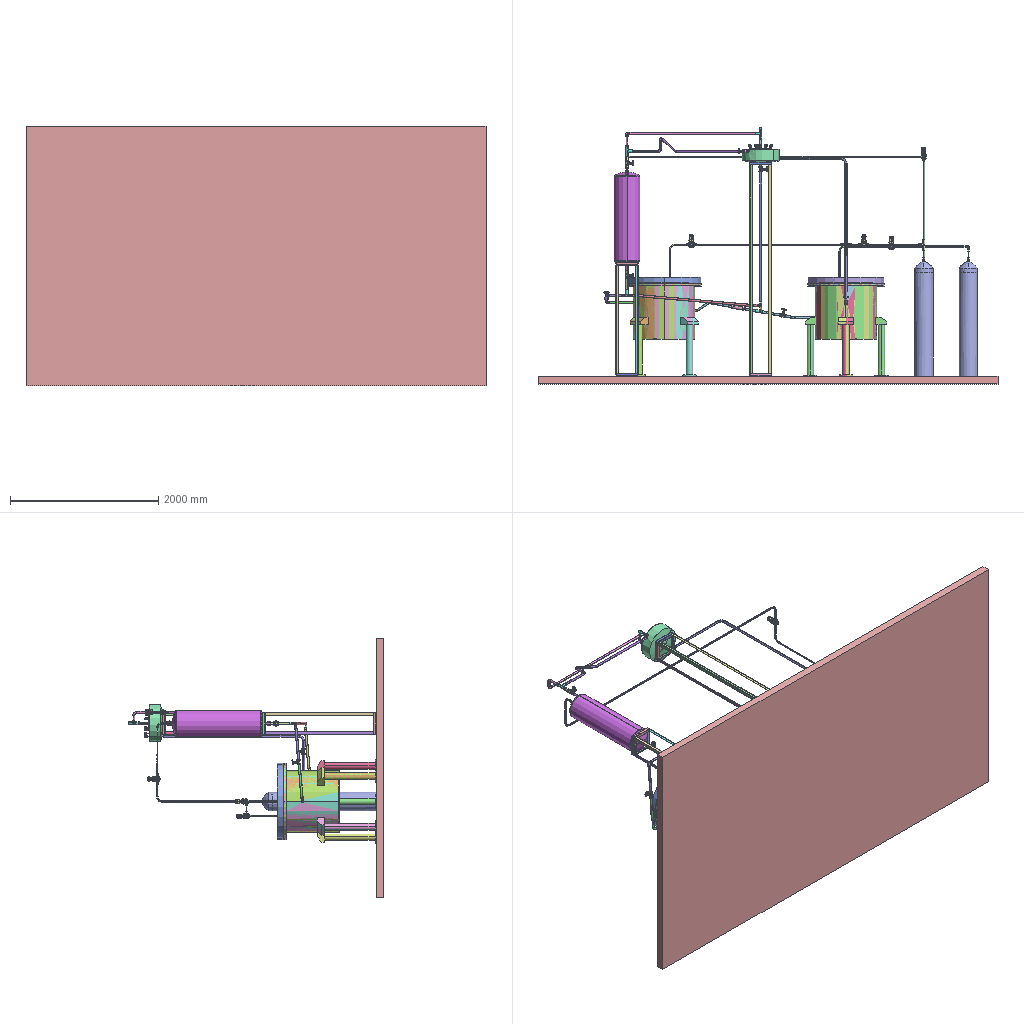Assembly | SolidWorks | 42 different items | 104 placed | box 6200 x 3449 x 3500 mm
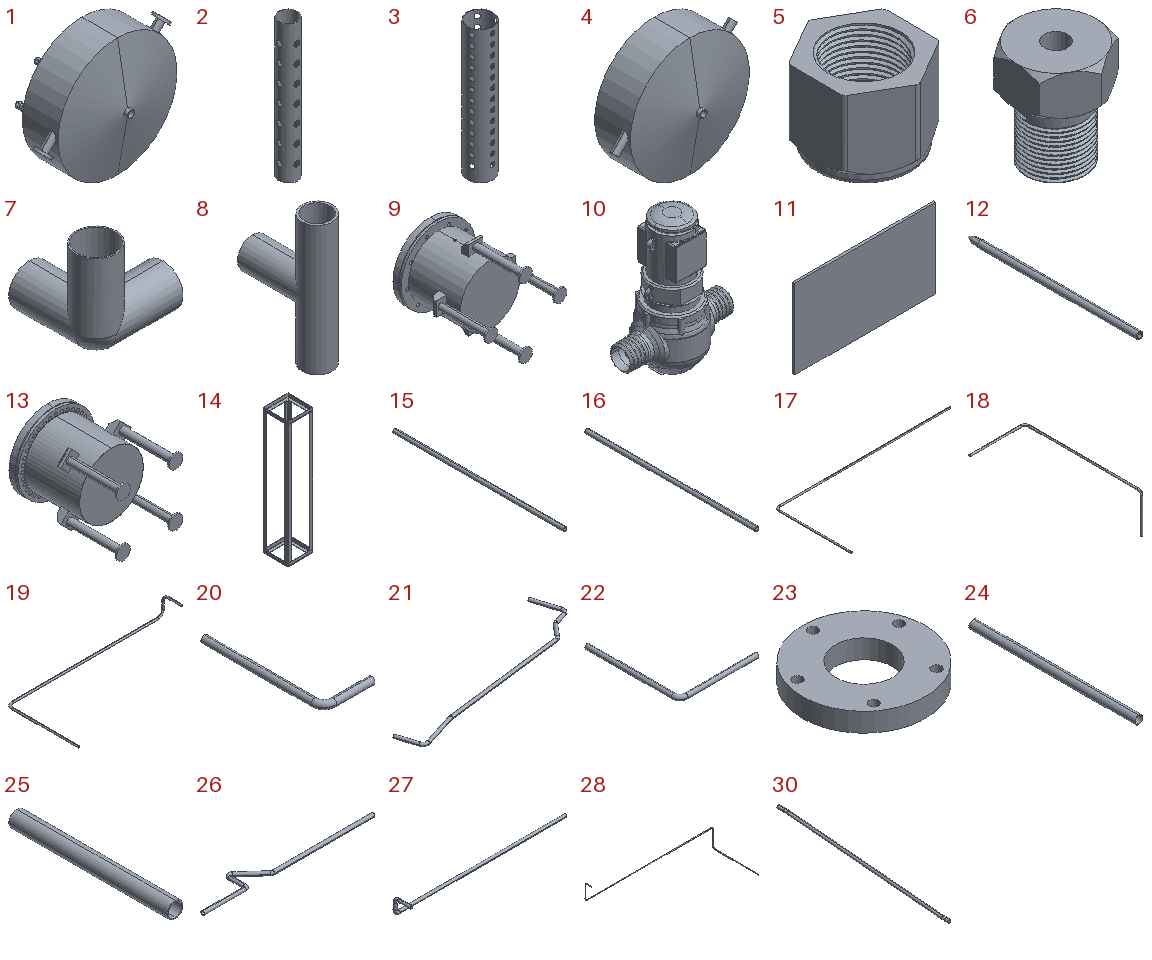Parts list (item | name | quantity | parent item | size | volume | features):
1 | (subassembly) | x1 | - | 652.028 x 361.167 x 500 mm | 2508772 mm3 | features ReferencePattern 8, LocalLPattern 2, 3DProfileFeature 1
2 | - | x14 | in 1 | 16 x 16 x 120 mm | 2633 mm3 | features BaseBody 1
3 | - | x1 | in 1 | 27 x 27 x 140 mm | 5187 mm3 | features BaseBody 1
4 | - | x1 | in 1 | - | - | features ICE 2, BaseBody 1, FillRefSurface 1
5 | - | x14 | in 1 | 20 x 22.785 x 17 mm | 3287 mm3 | features BaseBody 1
6 | - | x14 | in 1 | 20 x 23.094 x 26 mm | 5258 mm3 | features BaseBody 1
7 | - | x1 | - | - | - | features ICE 2, BaseBody 1, RefSurface 1
8 | - | x4 | - | 35 x 92.5 x 150 mm | 52141 mm3 | features BaseBody 1
9 | - | x1 | - | 1141 x 1336 x 1141 mm | 298249158 mm3 | features ICE 10, CirPattern 2, 3DProfileFeature 1, Extrusion 1, Shell 1
10 | - | x4 | - | - | - | features RefSurface 14, BaseBody 6, DelFace 5, Scale 1
11 | - | x1 | - | 6200 x 100 x 3500 mm | 2170000000 mm3 | features Cut 1, Extrusion 1
12 | - | x1 | in 1 | 6 x 151 x 6 mm | 2416 mm3 | features BaseBody 1
13 | - | x1 | - | 1000 x 1336 x 1000 mm | 288874329 mm3 | features ICE 9, CirPattern 2, Extrusion 1, Shell 1
14 | - | x1 | - | 300 x 300 x 1540 mm | 1903536 mm3 | features WeldMemberFeat 2, 3DProfileFeature 1, WeldmentFeature 1
15 | - | x1 | - | 20 x 900 x 20 mm | 101788 mm3 | features Sweep 1
16 | - | x1 | - | 20 x 800 x 20 mm | 90478 mm3 | features Sweep 1
17 | - | x1 | - | 2310 x 1010 x 20 mm | 370309 mm3 | features Sweep 1
18 | - | x1 | - | 936.356 x 1980 x 658.195 mm | 609287 mm3 | features 3DProfileFeature 2, Sweep 1
19 | - | x1 | - | 1755 x 810 x 220 mm | 676261 mm3 | features 3DProfileFeature 2, Sweep 1
20 | - | x1 | - | 215 x 517 x 30 mm | 120482 mm3 | features Sweep 1
21 | - | x1 | - | 1894 x 737.142 x 42.475 mm | 941942 mm3 | features 3DProfileFeature 2, Sweep 1
22 | - | x1 | - | 515 x 615 x 30 mm | 190502 mm3 | features Sweep 1
23 | - | x2 | in 1 | 65 x 65 x 10 mm | 25133 mm3 | features BaseBody 1
24 | - | x1 | - | 30 x 600 x 30 mm | 54664 mm3 | features Sweep 1
25 | - | x1 | - | 30 x 300 x 30 mm | 52779 mm3 | features Sweep 1
26 | - | x1 | - | 1430 x 195.048 x 30 mm | 288468 mm3 | features 3DProfileFeature 2, Sweep 1
27 | - | x1 | - | 1817 x 186.765 x 176.777 mm | 367085 mm3 | features 3DProfileFeature 2, Sweep 1
28 | - | x1 | - | 4020 x 1445 x 1070 mm | 1547370 mm3 | features 3DProfileFeature 2, Sweep 1
29 | - | x1 | - | - | - | features 3DProfileFeature 2, Sweep 1
30 | - | x1 | - | 30 x 1694 x 166.835 mm | 299072 mm3 | features 3DProfileFeature 2, Sweep 1
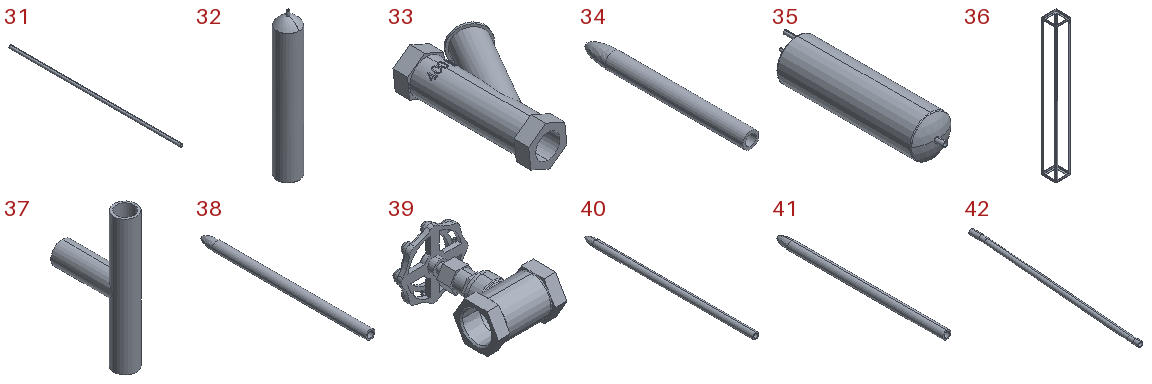31 | - | x1 | - | 30 x 1846 x 30 mm | 324836 mm3 | features Sweep 1
32 | - | x2 | - | - | - | features BaseBody 2, Fillet 1, ICE 1, RefSurface 1, RevCut 1, Shell 1
33 | - | x1 | - | 104.725 x 170.486 x 51.675 mm | 233814 mm3 | features ICE 5, Emboss 1, Extrusion 1, Scale 1, Sweep 1
34 | - | x3 | in 1 | 6 x 61 x 6 mm | 1002 mm3 | features BaseBody 1
35 | - | x1 | - | 350 x 1420 x 350 mm | 7280812 mm3 | features ICE 8, Revolution 1
36 | - | x1 | - | 300 x 300 x 2890 mm | 3177590 mm3 | features WeldMemberFeat 2, 3DProfileFeature 1, WeldmentFeature 1
37 | - | x2 | - | 25 x 82.626 x 150 mm | 36350 mm3 | features ICE 2, BaseBody 1
38 | - | x2 | in 1 | 6 x 111 x 6 mm | 1788 mm3 | features BaseBody 1
39 | - | x6 | - | 72 x 115.407 x 70 mm | 83947 mm3 | features BaseBody 1
40 | - | x4 | in 1 | 6 x 161 x 6 mm | 2573 mm3 | features BaseBody 1
41 | - | x4 | in 1 | 6 x 121 x 6 mm | 1945 mm3 | features BaseBody 1
42 | - | x1 | - | 30 x 1053 x 110.793 mm | 185949 mm3 | features 3DProfileFeature 2, Sweep 1
Mates (type | each side: item.copy, entity, surface, feature):
In the top assembly
Coincident | 11.1 face plane Boss-Extrude1 | 14.1 face plane GB/T9787-1988 Hot-rolled equal-leg angle steel 040 X 3(1)
Coincident | 11.1 face plane Boss-Extrude1 | 36.1 face plane GB/T9787-1988 Hot-rolled equal-leg angle steel 040 X 3(1)
Symmetric | 14.1 face plane GB/T9787-1988 Hot-rolled equal-leg angle steel 040 X 3(3) | 14.1 face plane GB/T9787-1988 Hot-rolled equal-leg angle steel 040 X 3(3) | 35.1 plane
Symmetric | 14.1 face plane GB/T9787-1988 Hot-rolled equal-leg angle steel 040 X 3(1) | 14.1 face plane GB/T9787-1988 Hot-rolled equal-leg angle steel 040 X 3(1) | 35.1 plane
Concentric | 35.1 face cylinder Boss-Extrude1 | 8.1 face cylinder Input1
Parallel | 8.1 plane | assembly plane
Coincident | 14.1 face plane GB/T9787-1988 Hot-rolled equal-leg angle steel 040 X 3(1) | 36.1 face plane GB/T9787-1988 Hot-rolled equal-leg angle steel 040 X 3(1)
DistanceDim | 13.1 plane | 11.1 face plane Boss-Extrude1 | 2 times
Parallel | 11.1 face plane Boss-Extrude1 | 39.1 plane
Coincident | 39.1 edge | 20.1 face plane Sweep-Thin1
Concentric | 20.1 face cylinder Sweep-Thin1 | 22.1 face cylinder Sweep-Thin1
Concentric | 35.1 face cylinder Boss-Extrude5 | 39.2 face cylinder Input1
Parallel | 14.1 face plane GB/T9787-1988 Hot-rolled equal-leg angle steel 040 X 3(1) | 39.2 plane
Concentric | 35.1 face cylinder Boss-Extrude5 | 8.2 face cylinder Input1
Parallel | 14.1 face plane GB/T9787-1988 Hot-rolled equal-leg angle steel 040 X 3(1) | 8.2 plane
Parallel | 36.1 face plane GB/T9787-1988 Hot-rolled equal-leg angle steel 040 X 3(3) | 8.3 plane
Concentric | 39.2 face cylinder Input1 | 25.1 face cylinder Sweep-Thin1
Coincident | 26.1 plane | assembly plane | 3 times
Coincident | 27.1 plane | assembly plane | 3 times
Coincident | 32.1 plane | 32.2 plane
Concentric | 10.1 face cylinder Product-2-surface6 | 28.1 face cylinder Sweep-Thin1
Parallel | 11.1 face plane Boss-Extrude1 | 10.1 face plane Product-2-solid3
Concentric | 28.1 face cylinder Sweep-Thin1 | 37.1 face cylinder Input1
Concentric | 37.1 face cylinder Input1 | 37.2 face cylinder Input1
Parallel | 37.1 face plane Input1 | 37.2 face plane Cut-Extrude1
Concentric | 37.1 face cylinder Input1 | 15.1 face cylinder Sweep-Thin1
Coincident | 37.1 face plane Cut-Extrude1 | 15.1 edge
Coincident | 37.2 face plane Input1 | 15.1 face plane Sweep-Thin1
Concentric | 37.2 face cylinder Input1 | 16.1 face cylinder Sweep-Thin1
Coincident | 37.2 edge | 16.1 face plane Sweep-Thin1
DistanceDim | 11.1 face plane Boss-Extrude1 | 37.1 face plane Input1
Concentric | 15.1 face cylinder Sweep-Thin1 | 10.2 face cylinder Product-1-surface6
Parallel | 11.1 face plane Boss-Extrude1 | 10.2 plane
Coincident | 37.2 face plane Input1 | 17.1 face plane Sweep-Thin1
Concentric | 37.2 face cylinder Input1 | 17.1 face cylinder Sweep-Thin1
Concentric | 17.1 face cylinder Sweep-Thin1 | 10.3 face cylinder Product-1-surface6
Coincident | 10.2 face plane Product-2-solid3 | 10.3 face plane Product-2-solid3
Coincident | 18.1 plane | assembly plane | 3 times
Parallel | 36.1 face plane GB/T9787-1988 Hot-rolled equal-leg angle steel 040 X 3(1) | 39.3 face plane Input1
Coincident | 19.1 plane | assembly plane | 3 times
Concentric | 19.1 face cylinder Sweep-Thin1 | 10.4 face cylinder Product-1-surface6
Parallel | 11.1 face plane Boss-Extrude1 | 10.4 face plane Product-2-solid3
Concentric | 31.1 face cylinder Sweep-Thin1 | 39.4 face cylinder Input1
Parallel | 36.1 face plane GB/T9787-1988 Hot-rolled equal-leg angle steel 040 X 3(1) | 39.4 face plane Input1
Parallel | 11.1 face plane Boss-Extrude1 | 33.1 plane
Concentric | 35.1 face cylinder Boss-Extrude1 | 39.5 face cylinder Input1
Parallel | 14.1 face plane GB/T9787-1988 Hot-rolled equal-leg angle steel 040 X 3(1) | 39.5 face plane Input1
Parallel | 39.1 plane | 20.1 plane
Concentric | 8.1 face cylinder Input1 | 20.1 face cylinder Sweep-Thin1
Coincident | 8.1 face plane Input1 | 20.1 face plane Sweep-Thin1
Parallel | 20.1 plane | 22.1 plane
Parallel | 11.1 face plane Boss-Extrude1 | 30.1 plane
Coincident | 13.1 plane | 9.1 plane | 2 times
DistanceDim | 13.1 plane | 9.1 plane
Tangent | 35.1 face sphere Revolve1 | 14.1 face cylinder GB/T9787-1988 Hot-rolled equal-leg angle steel 040 X 3(3)
DistanceDim | 14.1 plane | 11.1 face plane Boss-Extrude1 | 2 times
DistanceDim | 36.1 plane | 14.1 plane
DistanceDim | 32.1 plane | 32.2 plane
Coincident | 11.1 face plane Boss-Extrude1 | 32.2 face plane Boss-Extrude1
Coincident | 11.1 face plane Boss-Extrude1 | 32.1 face plane Boss-Extrude1
Coincident | 11.1 face plane Boss-Extrude1 | 13.1 face plane CirPattern5
Concentric | 13.1 face cylinder Cut-Extrude4 | 22.1 face cylinder Sweep-Thin1
PlanarAngleDim | 22.1 plane | 11.1 face plane Boss-Extrude1
Concentric | 39.1 face cylinder Input1 | 22.1 face cylinder Sweep-Thin1
Concentric | 35.1 face cylinder Boss-Extrude1 | 24.1 face cylinder Sweep-Thin1
Coincident | 24.1 face plane Sweep-Thin1 | 8.1 face plane Input1
Concentric | 4.1 face cylinder Input1 | 31.1 face cylinder Sweep-Thin1
Coincident | 4.1 face plane Input1 | 31.1 face plane Sweep-Thin1
Concentric | 7.1 face cylinder Input1 | 31.1 face cylinder Sweep-Thin1
Coincident | 7.1 edge | 31.1 face plane Sweep-Thin1
Concentric | 4.1 face cylinder Input1 | 8.3 face cylinder Input1
Concentric | 28.1 face cylinder Sweep-Thin1 | 32.1 face cylinder Cut-Revolve1
Concentric | 8.4 face cylinder Input1 | 39.6 face cylinder Input1
Concentric | 7.1 face cylinder Input1 | 42.1 face cylinder Sweep-Thin1
Coincident | 7.1 face plane Cut-Extrude2 | 42.1 face plane Sweep-Thin1
Concentric | 8.4 face cylinder Input1 | 42.1 face cylinder Sweep-Thin1
Concentric | 8.4 face cylinder Input1 | 33.1 face cylinder Boss-Extrude1
Parallel | 36.1 face plane GB/T9787-1988 Hot-rolled equal-leg angle steel 040 X 3(3) | 23.1 face plane Input1
Parallel | 11.1 face plane Cut-Extrude1 | 32.2 plane
DistanceDim | 32.2 plane | 11.1 face plane Cut-Extrude1
Concentric | 4.1 face cylinder Boss-Extrude1 | 26.1 face cylinder Sweep-Thin1
Parallel | 11.1 face plane Boss-Extrude1 | 32.2 plane
Coincident | 8.4 face plane Input1 | 42.1 face plane Sweep-Thin1
Concentric | 18.1 face cylinder Sweep-Thin1 | 39.3 face cone Input1
PlanarAngleDim | 8.4 plane | 11.1 face plane Boss-Extrude1
In subassembly 1
Concentric | 4.2 face cylinder Boss-Extrude1 | 23.2 face cylinder Input1
Coincident | 4.2 face plane Boss-Extrude1 | 23.2 face plane Input1